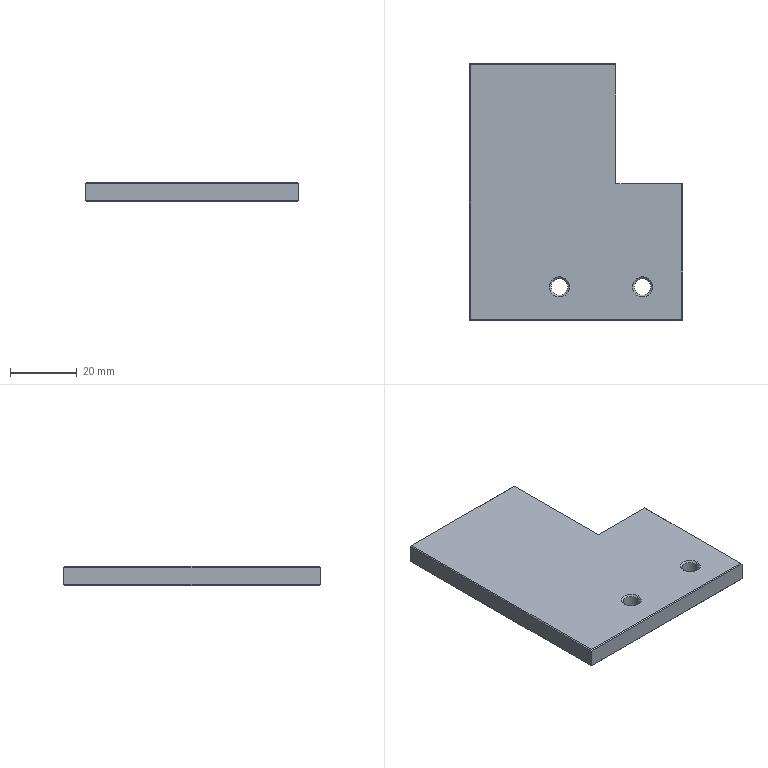Part | NX | 1 solid | 76 faces | box 64 x 77 x 6 mm | volume 24616 mm3 | cone 40 | cylinder 20 | plane 16 | commonest cylinder face diameters 2.5 x16 5 x4